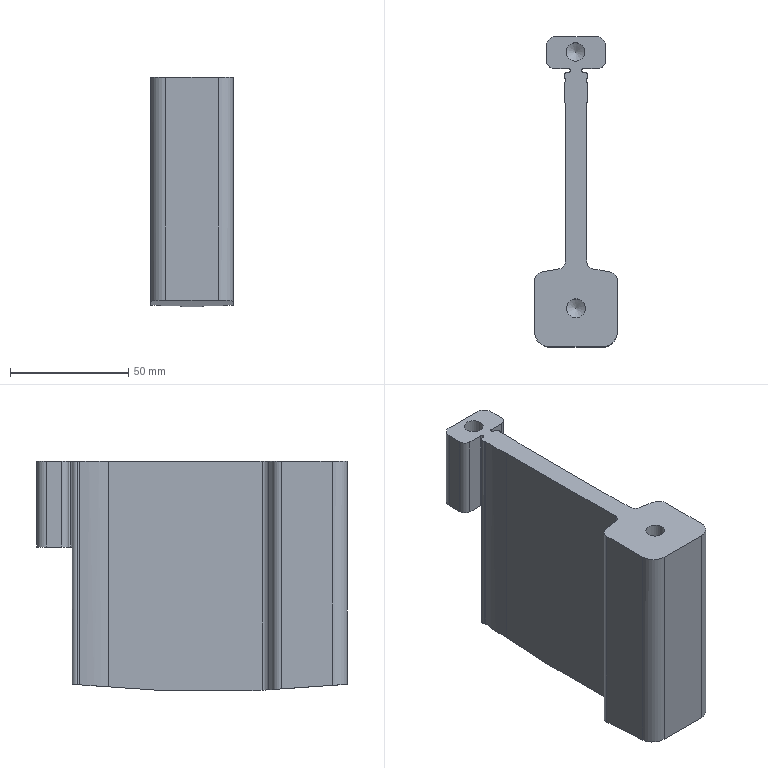Part | STEP file | 1_id146_x_t | 1 solid | 44 faces | box 35 x 131.5 x 97.111 mm | volume 189227 mm3 | cylinder 23 | plane 19 | cone 2 | commonest cylinder face diameters 1.5 x4 3 x4 6 x4 8 x4 7.938 x2 12.7 x2